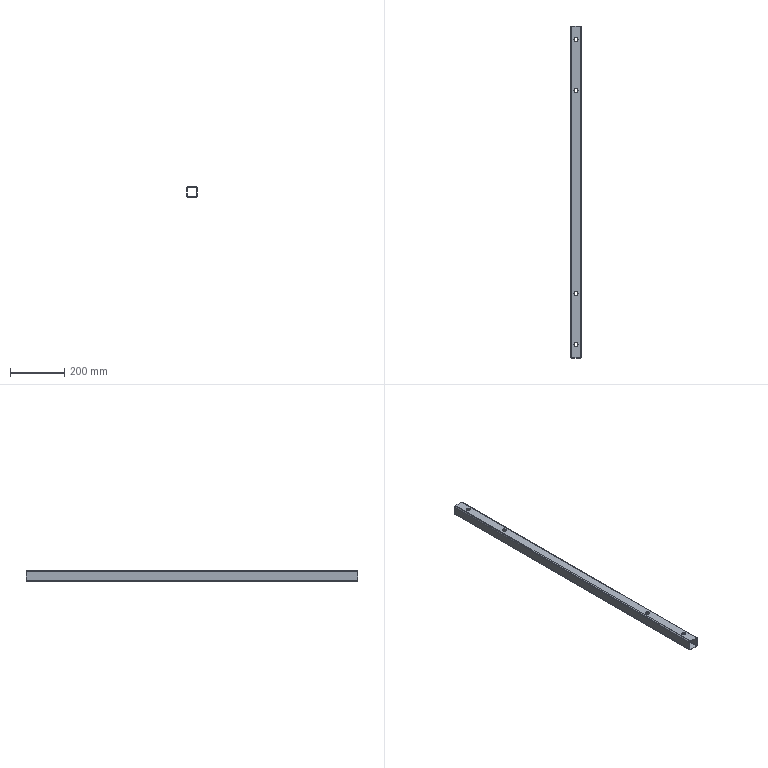Part | NX | features BREP 1 | 1 solid | 52 faces | box 40 x 1225 x 40 mm | volume 352740 mm3 | cylinder 28 | plane 24 | commonest cylinder face diameters 15 x16 6 x8 10 x4